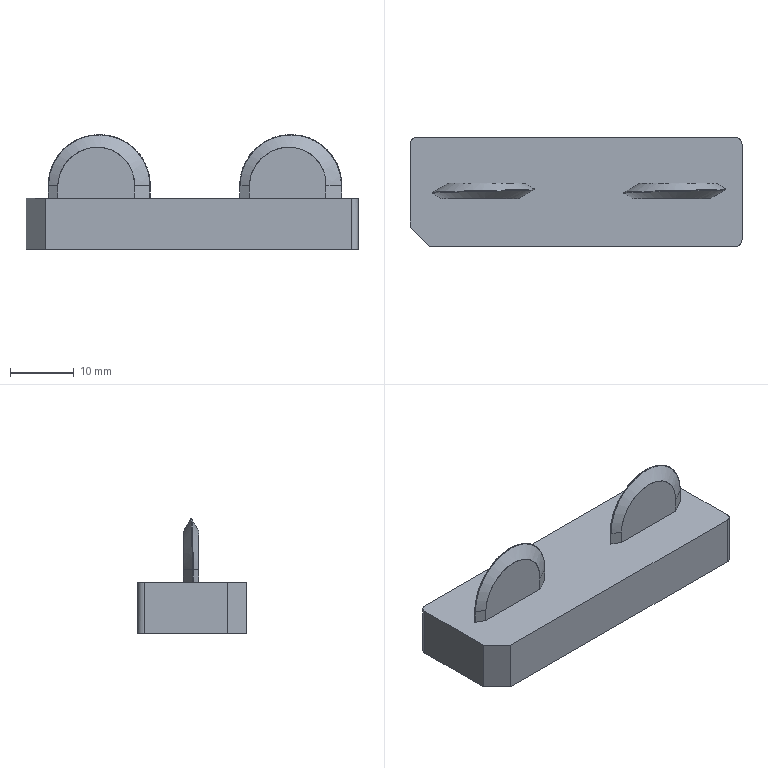CAM job | PowerMill | 3-axis milling, other | part box 52 x 17 x 17.993 mm
Tools:
number,name,type,diameter,tip_radius,length,cutting_length,overhang,flutes,holder,toolpaths_using
1,D10C,end_mill,10.0,0.0,60.0,,30.0,1,D42L35,1
1,D10C_1_1_1,end_mill,10.0,0.0,60.0,,18.44,1,D42L35,3
2,D4C_1_1,end_mill,4.0,0.0,30.0,,10.16,1,D42L35,1
3,D10_1_1_1,end_mill,10.0,0.0,60.0,,18.16,1,D42L35,2
4,R1_1_1,ball_nosed,2.0,1.0,3.8,,9.4,1,D42L35,1
10,D3_1_1,end_mill,3.0,0.0,30.0,,10.28,1,D42L35,1
13,Text_D4_1_1,taper_spherical,4.0,0.3,60.0,,10.24,1,D42L35,1
Operations:
program,toolpath,strategy,tool,tool_number,tool_diameter,tip_radius,flutes,spindle_rpm,feed_cut,surface_speed_m_min_computed,feed_per_tooth_computed,tolerance,thickness,stepover,stepdown,cut_length,cut_time_min,total_time_min,workplane
26-B01-0425-4-F,精公开粗01-扫面平行-D10C,raster_area_clear,D10C_1_1_1,1,10.0,0.0,1.0,8000.0,10000.0,251.33,1.25,0.03,0.3,6.0,1.0,310.6,0.031,0.0378,
26-B01-0425-4-F,精公开粗01-外形偏置-D10C,offset_area_clear,D10C_1_1_1,1,10.0,0.0,1.0,8000.0,10000.0,251.33,1.25,0.03,0.3,6.0,1.0,7861.677,0.786,0.85,
26-B01-0425-4-F,精公开粗01-基准台等高-D10C,constantz,D10C_1_1_1,1,10.0,0.0,1.0,8000.0,10000.0,251.33,1.25,0.03,0.07,5.0,0.4,3669.098,0.367,0.3771,
26-B01-0425-4-F,精公再粗02-外形偏置-D4C,offset_area_clear,D4C_1_1,2,4.0,0.0,1.0,18000.0,6000.0,226.19,0.3333,0.03,0.02,2.0,1.0,4187.404,0.698,0.7403,
26-B01-0425-4-F,精公基准台01-基准面偏置-D10,offset_area_clear,D10_1_1_1,3,10.0,0.0,1.0,8500.0,600.0,267.04,0.0706,0.005,0.4,5.0,1.0,177.683,0.296,0.3646,
26-B01-0425-4-F,精公基准台01-基准台侧光-D10,profile_area_clear,D10_1_1_1,3,10.0,0.0,1.0,8500.0,600.0,267.04,0.0706,0.005,0.0,0.08,1.0,333.233,0.555,0.6201,
26-B01-0425-4-F,精公精光01-浅滩和陡峭-R1,inter_constz,R1_1_1,4,2.0,1.0,1.0,18000.0,2000.0,113.1,0.1111,0.005,-0.055,0.03,1.0,11143.369,5.572,5.942,
26-B01-0425-4-F,精公精光02-等高-D3,constantz,D3_1_1,10,3.0,0.0,1.0,18000.0,2000.0,169.65,0.1111,0.005,-0.055,5.0,0.05,10615.323,5.308,5.678,
26-B01-0425-4-F,精公刻字01-刻字-Text_D4,pattern,Text_D4_1_1,13,4.0,0.3,1.0,15000.0,1000.0,188.5,0.0667,0.005,0.0,5.0,1.0,103.082,0.103,0.1283,
,精公开粗01-外形偏置-D10C_Reference,offset_area_clear,D10C,1,10.0,0.0,1.0,8000.0,10000.0,251.33,1.25,0.03,0.3,6.0,1.0,15729.522,1.573,1.697,